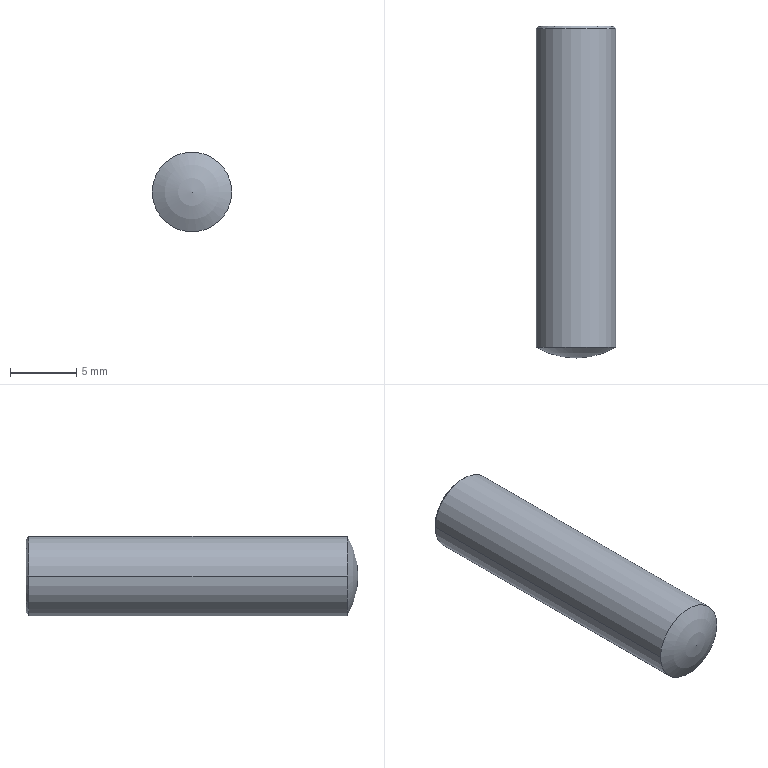Part | NX | 1 solid | 13 faces | box 6 x 25 x 6 mm | volume 672.015 mm3 | plane 8 | cylinder 2 | cone 2 | sphere 1 | commonest cylinder face diameters 6 x2
STEP:
#1=CARTESIAN_POINT('',(3.006,-25.2,0.000000001));
#2=VERTEX_POINT('',#1);
#3=CARTESIAN_POINT('',(-2.994,-25.2,0.000000001));
#4=VERTEX_POINT('',#3);
#5=CARTESIAN_POINT('',(0.006093,-25.2,0.000000001));
#6=DIRECTION('',(0.,-1.,0.));
#7=DIRECTION('',(-1.,0.,0.));
#8=AXIS2_PLACEMENT_3D('',#5,#6,#7);
#9=CIRCLE('',#8,3.);
#10=EDGE_CURVE('',#2,#4,#9,.T.);
#11=ORIENTED_EDGE('',*,*,#10,.T.);
#12=CARTESIAN_POINT('',(-2.994,-49.196,0.000000001));
#13=VERTEX_POINT('',#12);
#14=CARTESIAN_POINT('',(-2.994,-17.75,0.000000001));
#15=DIRECTION('',(0.,-1.,0.));
#16=VECTOR('',#15,1000.);
#17=LINE('',#14,#16);
#18=EDGE_CURVE('',#13,#4,#17,.F.);
#19=ORIENTED_EDGE('',*,*,#18,.F.);
#20=CARTESIAN_POINT('',(3.006,-49.196,0.000000001));
#21=VERTEX_POINT('',#20);
#22=CARTESIAN_POINT('',(0.006093,-49.196,0.000000001));
#23=DIRECTION('',(0.,-1.,0.));
#24=DIRECTION('',(-1.,0.,0.));
#25=AXIS2_PLACEMENT_3D('',#22,#23,#24);
#26=CIRCLE('',#25,3.);
#27=EDGE_CURVE('',#21,#13,#26,.T.);
#28=ORIENTED_EDGE('',*,*,#27,.F.);
#29=CARTESIAN_POINT('',(3.006,-17.75,0.000000001));
#30=DIRECTION('',(0.,-1.,0.));
#31=VECTOR('',#30,1000.);
#32=LINE('',#29,#31);
#33=EDGE_CURVE('',#21,#2,#32,.F.);
#34=ORIENTED_EDGE('',*,*,#33,.T.);
#35=EDGE_LOOP('',(#11,#19,#28,#34));
#36=FACE_BOUND('',#35,.T.);
#37=CARTESIAN_POINT('',(0.006093,-17.75,0.000000001));
#38=DIRECTION('',(0.,-1.,0.));
#39=DIRECTION('',(-1.,0.,0.));
#40=AXIS2_PLACEMENT_3D('',#37,#38,#39);
#41=CYLINDRICAL_SURFACE('',#40,3.);
#42=ADVANCED_FACE('',(#36),#41,.T.);
#43=CARTESIAN_POINT('',(0.006093,-49.196,0.000000001));
#44=DIRECTION('',(0.,-1.,0.));
#45=DIRECTION('',(-1.,0.,0.));
#46=AXIS2_PLACEMENT_3D('',#43,#44,#45);
#47=CIRCLE('',#46,3.);
#48=EDGE_CURVE('',#13,#21,#47,.T.);
#49=ORIENTED_EDGE('',*,*,#48,.T.);
#50=ORIENTED_EDGE('',*,*,#27,.T.);
#51=EDGE_LOOP('',(#49,#50));
#52=FACE_BOUND('',#51,.T.);
#53=CARTESIAN_POINT('',(0.006093,-44.,0.000000001));
#54=DIRECTION('',(0.,1.,0.));
#55=DIRECTION('',(1.,0.,0.));
#56=AXIS2_PLACEMENT_3D('',#53,#54,#55);
#57=SPHERICAL_SURFACE('',#56,6.);
#58=ADVANCED_FACE('',(#52),#57,.T.);
#59=CARTESIAN_POINT('',(-0.8599,-25.,1.5));
#60=VERTEX_POINT('',#59);
#61=CARTESIAN_POINT('',(-0.8599,-28.,1.5));
#62=VERTEX_POINT('',#61);
#63=CARTESIAN_POINT('',(-0.8599,0.,1.5));
#64=DIRECTION('',(0.,-1.,0.));
#65=VECTOR('',#64,1000.);
#66=LINE('',#63,#65);
#67=EDGE_CURVE('',#60,#62,#66,.T.);
#68=ORIENTED_EDGE('',*,*,#67,.F.);
#69=CARTESIAN_POINT('',(0.8721,-25.,1.5));
#70=VERTEX_POINT('',#69);
#71=CARTESIAN_POINT('',(0.,-25.,1.5));
#72=DIRECTION('',(-1.,0.,0.));
#73=VECTOR('',#72,1000.);
#74=LINE('',#71,#73);
#75=EDGE_CURVE('',#70,#60,#74,.T.);
#76=ORIENTED_EDGE('',*,*,#75,.F.);
#77=CARTESIAN_POINT('',(0.8721,-28.,1.5));
#78=VERTEX_POINT('',#77);
#79=CARTESIAN_POINT('',(0.8721,0.,1.5));
#80=DIRECTION('',(0.,1.,0.));
#81=VECTOR('',#80,1000.);
#82=LINE('',#79,#81);
#83=EDGE_CURVE('',#78,#70,#82,.T.);
#84=ORIENTED_EDGE('',*,*,#83,.F.);
#85=CARTESIAN_POINT('',(0.,-28.,1.5));
#86=DIRECTION('',(-1.,0.,0.));
#87=VECTOR('',#86,1000.);
#88=LINE('',#85,#87);
#89=EDGE_CURVE('',#78,#62,#88,.T.);
#90=ORIENTED_EDGE('',*,*,#89,.T.);
#91=EDGE_LOOP('',(#68,#76,#84,#90));
#92=FACE_BOUND('',#91,.T.);
#93=CARTESIAN_POINT('',(-0.8599,-25.,1.5));
#94=DIRECTION('',(0.,0.,1.));
#95=DIRECTION('',(1.,0.,0.));
#96=AXIS2_PLACEMENT_3D('',#93,#94,#95);
#97=PLANE('',#96);
#98=ADVANCED_FACE('',(#92),#97,.F.);
#99=CARTESIAN_POINT('',(1.738,-25.,0.000000001));
#100=VERTEX_POINT('',#99);
#101=CARTESIAN_POINT('',(1.738,-28.,0.000000001));
#102=VERTEX_POINT('',#101);
#103=CARTESIAN_POINT('',(1.738,0.,0.000000001));
#104=DIRECTION('',(0.,-1.,0.));
#105=VECTOR('',#104,1000.);
#106=LINE('',#103,#105);
#107=EDGE_CURVE('',#100,#102,#106,.T.);
#108=ORIENTED_EDGE('',*,*,#107,.F.);
#109=CARTESIAN_POINT('',(0.8721,-25.,-1.5));
#110=VERTEX_POINT('',#109);
#111=CARTESIAN_POINT('',(1.738,-25.,0.));
#112=DIRECTION('',(0.5,0.,0.866));
#113=VECTOR('',#112,1000.);
#114=LINE('',#111,#113);
#115=EDGE_CURVE('',#110,#100,#114,.T.);
#116=ORIENTED_EDGE('',*,*,#115,.F.);
#117=CARTESIAN_POINT('',(0.8721,-28.,-1.5));
#118=VERTEX_POINT('',#117);
#119=CARTESIAN_POINT('',(0.8721,0.,-1.5));
#120=DIRECTION('',(0.,1.,0.));
#121=VECTOR('',#120,1000.);
#122=LINE('',#119,#121);
#123=EDGE_CURVE('',#118,#110,#122,.T.);
#124=ORIENTED_EDGE('',*,*,#123,.F.);
#125=CARTESIAN_POINT('',(1.738,-28.,0.));
#126=DIRECTION('',(0.5,0.,0.866));
#127=VECTOR('',#126,1000.);
#128=LINE('',#125,#127);
#129=EDGE_CURVE('',#118,#102,#128,.T.);
#130=ORIENTED_EDGE('',*,*,#129,.T.);
#131=EDGE_LOOP('',(#108,#116,#124,#130));
#132=FACE_BOUND('',#131,.T.);
#133=CARTESIAN_POINT('',(1.738,-25.,0.000000001));
#134=DIRECTION('',(0.866,0.,-0.5));
#135=DIRECTION('',(0.,-1.,0.));
#136=AXIS2_PLACEMENT_3D('',#133,#134,#135);
#137=PLANE('',#136);
#138=ADVANCED_FACE('',(#132),#137,.F.);
#139=CARTESIAN_POINT('',(-2.794,-25.,0.000000001));
#140=VERTEX_POINT('',#139);
#141=CARTESIAN_POINT('',(2.806,-25.,0.000000001));
#142=VERTEX_POINT('',#141);
#143=CARTESIAN_POINT('',(0.006093,-25.,0.000000001));
#144=DIRECTION('',(0.,-1.,0.));
#145=DIRECTION('',(-1.,0.,0.));
#146=AXIS2_PLACEMENT_3D('',#143,#144,#145);
#147=CIRCLE('',#146,2.8);
#148=EDGE_CURVE('',#140,#142,#147,.T.);
#149=ORIENTED_EDGE('',*,*,#148,.T.);
#150=CARTESIAN_POINT('',(2.906,-25.1,0.000000001));
#151=DIRECTION('',(0.7071,-0.7071,0.));
#152=VECTOR('',#151,1000.);
#153=LINE('',#150,#152);
#154=EDGE_CURVE('',#142,#2,#153,.T.);
#155=ORIENTED_EDGE('',*,*,#154,.T.);
#156=CARTESIAN_POINT('',(0.006093,-25.2,0.000000001));
#157=DIRECTION('',(0.,-1.,0.));
#158=DIRECTION('',(-1.,0.,0.));
#159=AXIS2_PLACEMENT_3D('',#156,#157,#158);
#160=CIRCLE('',#159,3.);
#161=EDGE_CURVE('',#4,#2,#160,.T.);
#162=ORIENTED_EDGE('',*,*,#161,.F.);
#163=CARTESIAN_POINT('',(-2.894,-25.1,0.000000001));
#164=DIRECTION('',(-0.7071,-0.7071,0.));
#165=VECTOR('',#164,1000.);
#166=LINE('',#163,#165);
#167=EDGE_CURVE('',#140,#4,#166,.T.);
#168=ORIENTED_EDGE('',*,*,#167,.F.);
#169=EDGE_LOOP('',(#149,#155,#162,#168));
#170=FACE_BOUND('',#169,.T.);
#171=CARTESIAN_POINT('',(0.006093,-25.1,0.000000001));
#172=DIRECTION('',(0.,-1.,0.));
#173=DIRECTION('',(-1.,0.,0.));
#174=AXIS2_PLACEMENT_3D('',#171,#172,#173);
#175=CONICAL_SURFACE('',#174,2.9,0.7854);
#176=ADVANCED_FACE('',(#170),#175,.T.);
#177=ORIENTED_EDGE('',*,*,#148,.F.);
#178=CARTESIAN_POINT('',(0.006093,-25.,0.000000001));
#179=DIRECTION('',(0.,-1.,0.));
#180=DIRECTION('',(-1.,0.,0.));
#181=AXIS2_PLACEMENT_3D('',#178,#179,#180);
#182=CIRCLE('',#181,2.8);
#183=EDGE_CURVE('',#142,#140,#182,.T.);
#184=ORIENTED_EDGE('',*,*,#183,.F.);
#185=EDGE_LOOP('',(#177,#184));
#186=FACE_BOUND('',#185,.T.);
#187=CARTESIAN_POINT('',(-1.726,-25.,0.000000001));
#188=VERTEX_POINT('',#187);
#189=CARTESIAN_POINT('',(-0.8599,-25.,-1.5));
#190=VERTEX_POINT('',#189);
#191=CARTESIAN_POINT('',(-1.726,-25.,0.));
#192=DIRECTION('',(0.5,0.,-0.866));
#193=VECTOR('',#192,1000.);
#194=LINE('',#191,#193);
#195=EDGE_CURVE('',#188,#190,#194,.T.);
#196=ORIENTED_EDGE('',*,*,#195,.T.);
#197=CARTESIAN_POINT('',(0.,-25.,-1.5));
#198=DIRECTION('',(1.,0.,0.));
#199=VECTOR('',#198,1000.);
#200=LINE('',#197,#199);
#201=EDGE_CURVE('',#190,#110,#200,.T.);
#202=ORIENTED_EDGE('',*,*,#201,.T.);
#203=ORIENTED_EDGE('',*,*,#115,.T.);
#204=CARTESIAN_POINT('',(1.738,-25.,0.));
#205=DIRECTION('',(-0.5,0.,0.866));
#206=VECTOR('',#205,1000.);
#207=LINE('',#204,#206);
#208=EDGE_CURVE('',#100,#70,#207,.T.);
#209=ORIENTED_EDGE('',*,*,#208,.T.);
#210=ORIENTED_EDGE('',*,*,#75,.T.);
#211=CARTESIAN_POINT('',(-1.726,-25.,0.));
#212=DIRECTION('',(-0.5,0.,-0.866));
#213=VECTOR('',#212,1000.);
#214=LINE('',#211,#213);
#215=EDGE_CURVE('',#60,#188,#214,.T.);
#216=ORIENTED_EDGE('',*,*,#215,.T.);
#217=EDGE_LOOP('',(#196,#202,#203,#209,#210,#216));
#218=FACE_BOUND('',#217,.T.);
#219=CARTESIAN_POINT('',(0.006093,-25.,0.000000001));
#220=DIRECTION('',(0.,-1.,0.));
#221=DIRECTION('',(0.,0.,-1.));
#222=AXIS2_PLACEMENT_3D('',#219,#220,#221);
#223=PLANE('',#222);
#224=ADVANCED_FACE('',(#186,#218),#223,.F.);
#225=ORIENTED_EDGE('',*,*,#83,.T.);
#226=ORIENTED_EDGE('',*,*,#208,.F.);
#227=ORIENTED_EDGE('',*,*,#107,.T.);
#228=CARTESIAN_POINT('',(1.738,-28.,0.));
#229=DIRECTION('',(0.5,0.,-0.866));
#230=VECTOR('',#229,1000.);
#231=LINE('',#228,#230);
#232=EDGE_CURVE('',#78,#102,#231,.T.);
#233=ORIENTED_EDGE('',*,*,#232,.F.);
#234=EDGE_LOOP('',(#225,#226,#227,#233));
#235=FACE_BOUND('',#234,.T.);
#236=CARTESIAN_POINT('',(0.8721,-25.,1.5));
#237=DIRECTION('',(0.866,0.,0.5));
#238=DIRECTION('',(0.,-1.,0.));
#239=AXIS2_PLACEMENT_3D('',#236,#237,#238);
#240=PLANE('',#239);
#241=ADVANCED_FACE('',(#235),#240,.F.);
#242=CARTESIAN_POINT('',(-1.726,-28.,0.000000001));
#243=VERTEX_POINT('',#242);
#244=CARTESIAN_POINT('',(-1.726,0.,0.000000001));
#245=DIRECTION('',(0.,1.,0.));
#246=VECTOR('',#245,1000.);
#247=LINE('',#244,#246);
#248=EDGE_CURVE('',#243,#188,#247,.T.);
#249=ORIENTED_EDGE('',*,*,#248,.F.);
#250=CARTESIAN_POINT('',(-0.8599,-28.,-1.5));
#251=VERTEX_POINT('',#250);
#252=CARTESIAN_POINT('',(-1.726,-28.,0.));
#253=DIRECTION('',(0.5,0.,-0.866));
#254=VECTOR('',#253,1000.);
#255=LINE('',#252,#254);
#256=EDGE_CURVE('',#243,#251,#255,.T.);
#257=ORIENTED_EDGE('',*,*,#256,.T.);
#258=CARTESIAN_POINT('',(-0.8599,0.,-1.5));
#259=DIRECTION('',(0.,-1.,0.));
#260=VECTOR('',#259,1000.);
#261=LINE('',#258,#260);
#262=EDGE_CURVE('',#190,#251,#261,.T.);
#263=ORIENTED_EDGE('',*,*,#262,.F.);
#264=ORIENTED_EDGE('',*,*,#195,.F.);
#265=EDGE_LOOP('',(#249,#257,#263,#264));
#266=FACE_BOUND('',#265,.T.);
#267=CARTESIAN_POINT('',(-0.8599,-25.,-1.5));
#268=DIRECTION('',(-0.866,0.,-0.5));
#269=DIRECTION('',(-0.5,0.,0.866));
#270=AXIS2_PLACEMENT_3D('',#267,#268,#269);
#271=PLANE('',#270);
#272=ADVANCED_FACE('',(#266),#271,.F.);
#273=ORIENTED_EDGE('',*,*,#248,.T.);
#274=ORIENTED_EDGE('',*,*,#215,.F.);
#275=ORIENTED_EDGE('',*,*,#67,.T.);
#276=CARTESIAN_POINT('',(-1.726,-28.,0.));
#277=DIRECTION('',(-0.5,0.,-0.866));
#278=VECTOR('',#277,1000.);
#279=LINE('',#276,#278);
#280=EDGE_CURVE('',#62,#243,#279,.T.);
#281=ORIENTED_EDGE('',*,*,#280,.T.);
#282=EDGE_LOOP('',(#273,#274,#275,#281));
#283=FACE_BOUND('',#282,.T.);
#284=CARTESIAN_POINT('',(-1.726,-25.,0.000000001));
#285=DIRECTION('',(-0.866,0.,0.5));
#286=DIRECTION('',(0.,1.,0.));
#287=AXIS2_PLACEMENT_3D('',#284,#285,#286);
#288=PLANE('',#287);
#289=ADVANCED_FACE('',(#283),#288,.F.);
#290=ORIENTED_EDGE('',*,*,#256,.F.);
#291=ORIENTED_EDGE('',*,*,#280,.F.);
#292=ORIENTED_EDGE('',*,*,#89,.F.);
#293=ORIENTED_EDGE('',*,*,#232,.T.);
#294=ORIENTED_EDGE('',*,*,#129,.F.);
#295=CARTESIAN_POINT('',(0.,-28.,-1.5));
#296=DIRECTION('',(1.,0.,0.));
#297=VECTOR('',#296,1000.);
#298=LINE('',#295,#297);
#299=EDGE_CURVE('',#251,#118,#298,.T.);
#300=ORIENTED_EDGE('',*,*,#299,.F.);
#301=EDGE_LOOP('',(#290,#291,#292,#293,#294,#300));
#302=FACE_BOUND('',#301,.T.);
#303=CARTESIAN_POINT('',(0.006093,-28.,0.000000001));
#304=DIRECTION('',(0.,1.,0.));
#305=DIRECTION('',(1.,0.,0.));
#306=AXIS2_PLACEMENT_3D('',#303,#304,#305);
#307=PLANE('',#306);
#308=ADVANCED_FACE('',(#302),#307,.T.);
#309=ORIENTED_EDGE('',*,*,#123,.T.);
#310=ORIENTED_EDGE('',*,*,#201,.F.);
#311=ORIENTED_EDGE('',*,*,#262,.T.);
#312=ORIENTED_EDGE('',*,*,#299,.T.);
#313=EDGE_LOOP('',(#309,#310,#311,#312));
#314=FACE_BOUND('',#313,.T.);
#315=CARTESIAN_POINT('',(0.8721,-25.,-1.5));
#316=DIRECTION('',(0.,0.,-1.));
#317=DIRECTION('',(0.,-1.,0.));
#318=AXIS2_PLACEMENT_3D('',#315,#316,#317);
#319=PLANE('',#318);
#320=ADVANCED_FACE('',(#314),#319,.F.);
#321=ORIENTED_EDGE('',*,*,#10,.F.);
#322=ORIENTED_EDGE('',*,*,#154,.F.);
#323=ORIENTED_EDGE('',*,*,#183,.T.);
#324=ORIENTED_EDGE('',*,*,#167,.T.);
#325=EDGE_LOOP('',(#321,#322,#323,#324));
#326=FACE_BOUND('',#325,.T.);
#327=CARTESIAN_POINT('',(0.006093,-25.1,0.000000001));
#328=DIRECTION('',(0.,-1.,0.));
#329=DIRECTION('',(-1.,0.,0.));
#330=AXIS2_PLACEMENT_3D('',#327,#328,#329);
#331=CONICAL_SURFACE('',#330,2.9,0.7854);
#332=ADVANCED_FACE('',(#326),#331,.T.);
#333=ORIENTED_EDGE('',*,*,#48,.F.);
#334=ORIENTED_EDGE('',*,*,#18,.T.);
#335=ORIENTED_EDGE('',*,*,#161,.T.);
#336=ORIENTED_EDGE('',*,*,#33,.F.);
#337=EDGE_LOOP('',(#333,#334,#335,#336));
#338=FACE_BOUND('',#337,.T.);
#339=CARTESIAN_POINT('',(0.006093,-17.75,0.000000001));
#340=DIRECTION('',(0.,-1.,0.));
#341=DIRECTION('',(-1.,0.,0.));
#342=AXIS2_PLACEMENT_3D('',#339,#340,#341);
#343=CYLINDRICAL_SURFACE('',#342,3.);
#344=ADVANCED_FACE('',(#338),#343,.T.);
#345=CLOSED_SHELL('',(#42,#58,#98,#138,#176,#224,#241,#272,#289,#308,#320,#332,#344));
#346=MANIFOLD_SOLID_BREP('',#345);
#347=(LENGTH_UNIT()NAMED_UNIT(*)SI_UNIT(.MILLI.,.METRE.));
#348=UNCERTAINTY_MEASURE_WITH_UNIT(LENGTH_MEASURE(0.00001),#347,'','');
#349=(NAMED_UNIT(*)PLANE_ANGLE_UNIT()SI_UNIT($,.RADIAN.));
#350=(NAMED_UNIT(*)SI_UNIT($,.STERADIAN.)SOLID_ANGLE_UNIT());
#351=(GEOMETRIC_REPRESENTATION_CONTEXT(3)GLOBAL_UNCERTAINTY_ASSIGNED_CONTEXT((#348))GLOBAL_UNIT_ASSIGNED_CONTEXT((#347,#349,#350))REPRESENTATION_CONTEXT('',''));
#352=ADVANCED_BREP_SHAPE_REPRESENTATION('',(#346),#351);